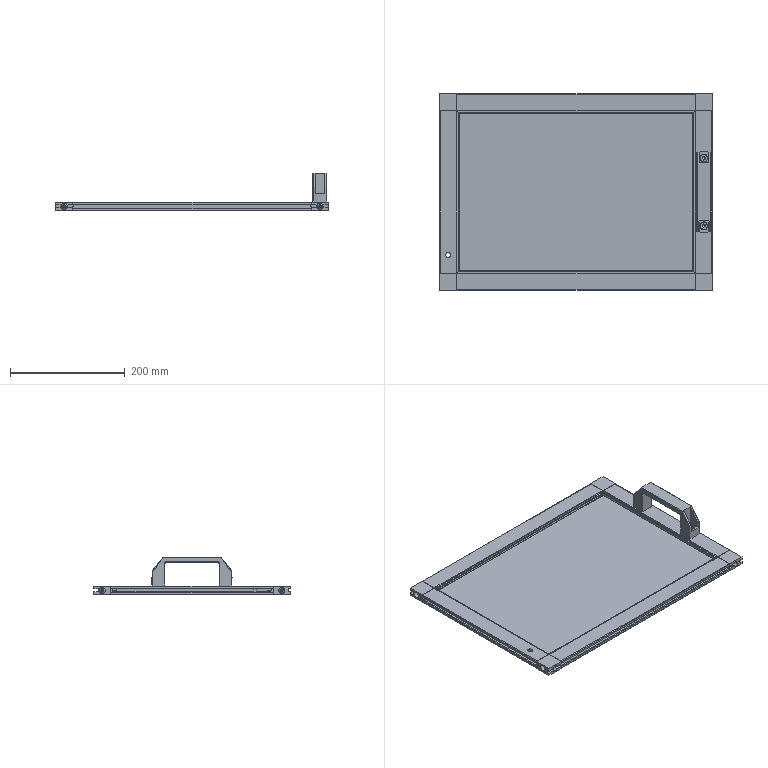Part | NX | features BREP 11 | 24 solids | 904 faces | box 475 x 342 x 65 mm | volume 835446 mm3 | plane 572 | cylinder 240 | cone 44 | torus 40 | spline 4 | sphere 4 | commonest cylinder face diameters 1 x42 5 x35 2 x32 11 x32 0.4 x24 6 x18